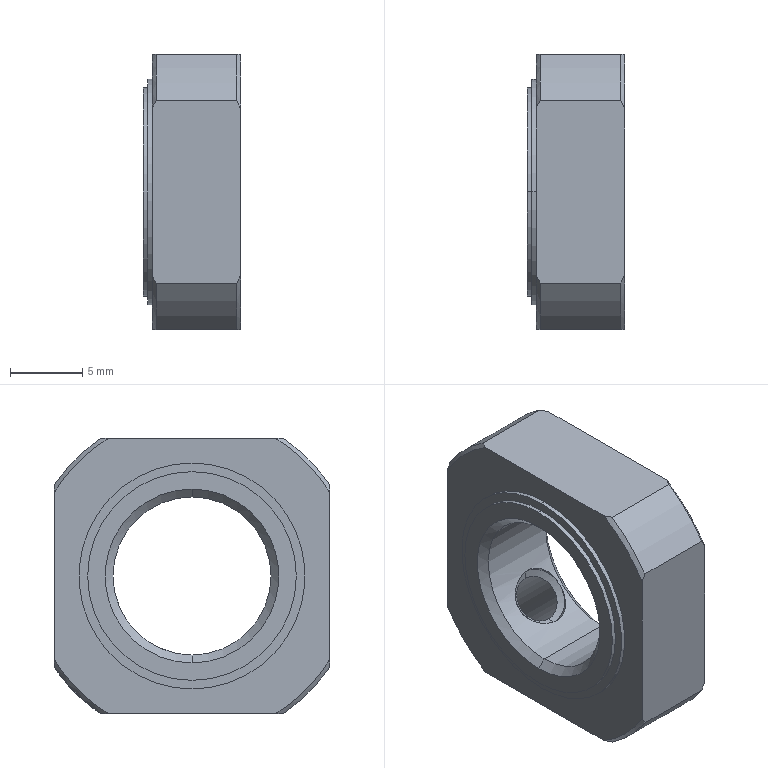Part | STEP file | 12bswnut | 1 solid | 39 faces | box 6.7 x 19 x 19 mm | volume 1510 mm3 | cone 16 | cylinder 15 | plane 8 | commonest cylinder face diameters 22.8 x4 4 x3 3.242 x2 10.917 x2 14.4 x2 15.6 x2
STEP:
#1=CARTESIAN_POINT('',(6.159,0.,-5.458));
#2=VERTEX_POINT('',#1);
#3=CARTESIAN_POINT('',(6.159,0.,5.458));
#4=VERTEX_POINT('',#3);
#5=CARTESIAN_POINT('',(6.159,0.,0.));
#6=DIRECTION('',(-1.,0.,0.));
#7=DIRECTION('',(0.,0.,1.));
#8=AXIS2_PLACEMENT_3D('',#5,#6,#7);
#9=CIRCLE('',#8,5.458);
#10=EDGE_CURVE('',#2,#4,#9,.T.);
#11=ORIENTED_EDGE('',*,*,#10,.T.);
#12=CARTESIAN_POINT('',(6.7,0.,6.));
#13=VERTEX_POINT('',#12);
#14=CARTESIAN_POINT('',(6.7,0.,6.));
#15=DIRECTION('',(0.7071,0.,0.7071));
#16=VECTOR('',#15,1000.);
#17=LINE('',#14,#16);
#18=EDGE_CURVE('',#4,#13,#17,.T.);
#19=ORIENTED_EDGE('',*,*,#18,.T.);
#20=CARTESIAN_POINT('',(6.7,0.,-6.));
#21=VERTEX_POINT('',#20);
#22=CARTESIAN_POINT('',(6.7,0.,0.));
#23=DIRECTION('',(-1.,0.,0.));
#24=DIRECTION('',(0.,0.,1.));
#25=AXIS2_PLACEMENT_3D('',#22,#23,#24);
#26=CIRCLE('',#25,6.);
#27=EDGE_CURVE('',#21,#13,#26,.T.);
#28=ORIENTED_EDGE('',*,*,#27,.F.);
#29=CARTESIAN_POINT('',(6.7,0.,-6.));
#30=DIRECTION('',(0.7071,0.,-0.7071));
#31=VECTOR('',#30,1000.);
#32=LINE('',#29,#31);
#33=EDGE_CURVE('',#2,#21,#32,.T.);
#34=ORIENTED_EDGE('',*,*,#33,.F.);
#35=EDGE_LOOP('',(#11,#19,#28,#34));
#36=FACE_OUTER_BOUND('',#35,.T.);
#37=CARTESIAN_POINT('',(6.7,0.,0.));
#38=DIRECTION('',(1.,0.,0.));
#39=DIRECTION('',(0.,0.,-1.));
#40=AXIS2_PLACEMENT_3D('',#37,#38,#39);
#41=CONICAL_SURFACE('',#40,6.,0.7854);
#42=ADVANCED_FACE('',(#36),#41,.F.);
#43=ORIENTED_EDGE('',*,*,#10,.F.);
#44=CARTESIAN_POINT('',(0.5415,0.,-5.458));
#45=VERTEX_POINT('',#44);
#46=CARTESIAN_POINT('',(6.7,0.,-5.458));
#47=DIRECTION('',(-1.,0.,0.));
#48=VECTOR('',#47,1000.);
#49=LINE('',#46,#48);
#50=EDGE_CURVE('',#2,#45,#49,.T.);
#51=ORIENTED_EDGE('',*,*,#50,.T.);
#52=CARTESIAN_POINT('',(0.5415,0.,5.458));
#53=VERTEX_POINT('',#52);
#54=CARTESIAN_POINT('',(0.5415,0.,0.));
#55=DIRECTION('',(-1.,0.,0.));
#56=DIRECTION('',(0.,0.,1.));
#57=AXIS2_PLACEMENT_3D('',#54,#55,#56);
#58=CIRCLE('',#57,5.458);
#59=EDGE_CURVE('',#45,#53,#58,.T.);
#60=ORIENTED_EDGE('',*,*,#59,.T.);
#61=CARTESIAN_POINT('',(6.7,0.,5.458));
#62=DIRECTION('',(-1.,0.,0.));
#63=VECTOR('',#62,1000.);
#64=LINE('',#61,#63);
#65=EDGE_CURVE('',#4,#53,#64,.T.);
#66=ORIENTED_EDGE('',*,*,#65,.F.);
#67=EDGE_LOOP('',(#43,#51,#60,#66));
#68=FACE_OUTER_BOUND('',#67,.T.);
#69=CARTESIAN_POINT('',(6.7,0.,0.));
#70=DIRECTION('',(-1.,0.,0.));
#71=DIRECTION('',(0.,0.,1.));
#72=AXIS2_PLACEMENT_3D('',#69,#70,#71);
#73=CYLINDRICAL_SURFACE('',#72,5.458);
#74=ADVANCED_FACE('',(#68),#73,.F.);
#75=ORIENTED_EDGE('',*,*,#59,.F.);
#76=CARTESIAN_POINT('',(0.,0.,-6.));
#77=VERTEX_POINT('',#76);
#78=CARTESIAN_POINT('',(0.5415,0.,-5.458));
#79=DIRECTION('',(-0.7071,0.,-0.7071));
#80=VECTOR('',#79,1000.);
#81=LINE('',#78,#80);
#82=EDGE_CURVE('',#45,#77,#81,.T.);
#83=ORIENTED_EDGE('',*,*,#82,.T.);
#84=CARTESIAN_POINT('',(0.,0.,6.));
#85=VERTEX_POINT('',#84);
#86=CARTESIAN_POINT('',(0.,0.,0.));
#87=DIRECTION('',(-1.,0.,0.));
#88=DIRECTION('',(0.,0.,1.));
#89=AXIS2_PLACEMENT_3D('',#86,#87,#88);
#90=CIRCLE('',#89,6.);
#91=EDGE_CURVE('',#77,#85,#90,.T.);
#92=ORIENTED_EDGE('',*,*,#91,.T.);
#93=CARTESIAN_POINT('',(0.5415,0.,5.458));
#94=DIRECTION('',(-0.7071,0.,0.7071));
#95=VECTOR('',#94,1000.);
#96=LINE('',#93,#95);
#97=EDGE_CURVE('',#53,#85,#96,.T.);
#98=ORIENTED_EDGE('',*,*,#97,.F.);
#99=EDGE_LOOP('',(#75,#83,#92,#98));
#100=FACE_OUTER_BOUND('',#99,.T.);
#101=CARTESIAN_POINT('',(0.5415,0.,0.));
#102=DIRECTION('',(-1.,0.,0.));
#103=DIRECTION('',(0.,0.,1.));
#104=AXIS2_PLACEMENT_3D('',#101,#102,#103);
#105=CONICAL_SURFACE('',#104,5.458,0.7854);
#106=ADVANCED_FACE('',(#100),#105,.F.);
#107=CARTESIAN_POINT('',(3.95,2.982,-5.274));
#108=VERTEX_POINT('',#107);
#109=CARTESIAN_POINT('',(3.95,5.274,-2.982));
#110=VERTEX_POINT('',#109);
#111=CARTESIAN_POINT('',(3.95,4.128,-4.128));
#112=DIRECTION('',(0.,0.7071,-0.7071));
#113=DIRECTION('',(0.,0.7071,0.7071));
#114=AXIS2_PLACEMENT_3D('',#111,#112,#113);
#115=CIRCLE('',#114,1.621);
#116=EDGE_CURVE('',#108,#110,#115,.T.);
#117=ORIENTED_EDGE('',*,*,#116,.T.);
#118=CARTESIAN_POINT('',(3.95,5.274,-2.446));
#119=VERTEX_POINT('',#118);
#120=CARTESIAN_POINT('',(3.95,5.274,-2.446));
#121=DIRECTION('',(0.,0.,1.));
#122=VECTOR('',#121,1000.);
#123=LINE('',#120,#122);
#124=EDGE_CURVE('',#110,#119,#123,.T.);
#125=ORIENTED_EDGE('',*,*,#124,.T.);
#126=CARTESIAN_POINT('',(1.95,3.86,-3.86));
#127=VERTEX_POINT('',#126);
#128=CARTESIAN_POINT('',(3.95,3.86,-3.86));
#129=DIRECTION('',(0.,0.7071,-0.7071));
#130=DIRECTION('',(0.,0.7071,0.7071));
#131=AXIS2_PLACEMENT_3D('',#128,#129,#130);
#132=CIRCLE('',#131,2.);
#133=EDGE_CURVE('',#127,#119,#132,.T.);
#134=ORIENTED_EDGE('',*,*,#133,.F.);
#135=CARTESIAN_POINT('',(3.95,2.446,-5.274));
#136=VERTEX_POINT('',#135);
#137=CARTESIAN_POINT('',(3.95,3.86,-3.86));
#138=DIRECTION('',(0.,0.7071,-0.7071));
#139=DIRECTION('',(0.,0.7071,0.7071));
#140=AXIS2_PLACEMENT_3D('',#137,#138,#139);
#141=CIRCLE('',#140,2.);
#142=EDGE_CURVE('',#136,#127,#141,.T.);
#143=ORIENTED_EDGE('',*,*,#142,.F.);
#144=CARTESIAN_POINT('',(3.95,2.446,-5.274));
#145=DIRECTION('',(0.,-1.,0.));
#146=VECTOR('',#145,1000.);
#147=LINE('',#144,#146);
#148=EDGE_CURVE('',#108,#136,#147,.T.);
#149=ORIENTED_EDGE('',*,*,#148,.F.);
#150=EDGE_LOOP('',(#117,#125,#134,#143,#149));
#151=FACE_OUTER_BOUND('',#150,.T.);
#152=CARTESIAN_POINT('',(3.95,3.86,-3.86));
#153=DIRECTION('',(0.,-0.7071,0.7071));
#154=DIRECTION('',(0.,-0.7071,-0.7071));
#155=AXIS2_PLACEMENT_3D('',#152,#153,#154);
#156=CONICAL_SURFACE('',#155,2.,0.7854);
#157=ADVANCED_FACE('',(#151),#156,.F.);
#158=ORIENTED_EDGE('',*,*,#116,.F.);
#159=CARTESIAN_POINT('',(3.95,6.647,-8.939));
#160=VERTEX_POINT('',#159);
#161=CARTESIAN_POINT('',(3.95,-1.146,-1.146));
#162=DIRECTION('',(0.,0.7071,-0.7071));
#163=VECTOR('',#162,1000.);
#164=LINE('',#161,#163);
#165=EDGE_CURVE('',#108,#160,#164,.T.);
#166=ORIENTED_EDGE('',*,*,#165,.T.);
#167=CARTESIAN_POINT('',(3.95,8.939,-6.647));
#168=VERTEX_POINT('',#167);
#169=CARTESIAN_POINT('',(3.95,7.793,-7.793));
#170=DIRECTION('',(0.,0.7071,-0.7071));
#171=DIRECTION('',(0.,0.7071,0.7071));
#172=AXIS2_PLACEMENT_3D('',#169,#170,#171);
#173=CIRCLE('',#172,1.621);
#174=EDGE_CURVE('',#160,#168,#173,.T.);
#175=ORIENTED_EDGE('',*,*,#174,.T.);
#176=CARTESIAN_POINT('',(3.95,1.146,1.146));
#177=DIRECTION('',(0.,0.7071,-0.7071));
#178=VECTOR('',#177,1000.);
#179=LINE('',#176,#178);
#180=EDGE_CURVE('',#110,#168,#179,.T.);
#181=ORIENTED_EDGE('',*,*,#180,.F.);
#182=EDGE_LOOP('',(#158,#166,#175,#181));
#183=FACE_OUTER_BOUND('',#182,.T.);
#184=CARTESIAN_POINT('',(3.95,0.,0.));
#185=DIRECTION('',(0.,0.7071,-0.7071));
#186=DIRECTION('',(0.,0.7071,0.7071));
#187=AXIS2_PLACEMENT_3D('',#184,#185,#186);
#188=CYLINDRICAL_SURFACE('',#187,1.621);
#189=ADVANCED_FACE('',(#183),#188,.F.);
#190=ORIENTED_EDGE('',*,*,#174,.F.);
#191=CARTESIAN_POINT('',(3.95,6.647,-9.262));
#192=VERTEX_POINT('',#191);
#193=CARTESIAN_POINT('',(3.95,6.647,-8.939));
#194=DIRECTION('',(0.,0.,-1.));
#195=VECTOR('',#194,1000.);
#196=LINE('',#193,#195);
#197=EDGE_CURVE('',#160,#192,#196,.T.);
#198=ORIENTED_EDGE('',*,*,#197,.T.);
#199=CARTESIAN_POINT('',(3.95,9.262,-6.647));
#200=VERTEX_POINT('',#199);
#201=CARTESIAN_POINT('',(3.95,6.647,-9.262));
#202=CARTESIAN_POINT('',(3.699,6.647,-9.262));
#203=CARTESIAN_POINT('',(3.445,6.684,-9.235));
#204=CARTESIAN_POINT('',(2.975,6.826,-9.131));
#205=CARTESIAN_POINT('',(2.753,6.932,-9.052));
#206=CARTESIAN_POINT('',(2.471,7.129,-8.896));
#207=CARTESIAN_POINT('',(2.384,7.203,-8.837));
#208=CARTESIAN_POINT('',(2.233,7.358,-8.708));
#209=CARTESIAN_POINT('',(2.168,7.44,-8.638));
#210=CARTESIAN_POINT('',(2.06,7.613,-8.486));
#211=CARTESIAN_POINT('',(2.02,7.702,-8.406));
#212=CARTESIAN_POINT('',(1.964,7.88,-8.239));
#213=CARTESIAN_POINT('',(1.95,7.972,-8.15));
#214=CARTESIAN_POINT('',(1.95,8.15,-7.972));
#215=CARTESIAN_POINT('',(1.964,8.237,-7.882));
#216=CARTESIAN_POINT('',(2.019,8.406,-7.702));
#217=CARTESIAN_POINT('',(2.061,8.487,-7.612));
#218=CARTESIAN_POINT('',(2.167,8.637,-7.441));
#219=CARTESIAN_POINT('',(2.233,8.708,-7.358));
#220=CARTESIAN_POINT('',(2.385,8.837,-7.202));
#221=CARTESIAN_POINT('',(2.47,8.895,-7.13));
#222=CARTESIAN_POINT('',(2.658,9.,-6.998));
#223=CARTESIAN_POINT('',(2.761,9.046,-6.938));
#224=CARTESIAN_POINT('',(2.977,9.124,-6.835));
#225=CARTESIAN_POINT('',(3.09,9.157,-6.791));
#226=CARTESIAN_POINT('',(3.447,9.236,-6.683));
#227=CARTESIAN_POINT('',(3.697,9.262,-6.647));
#228=CARTESIAN_POINT('',(3.95,9.262,-6.647));
#229=B_SPLINE_CURVE_WITH_KNOTS('',3,(#201,#202,#203,#204,#205,#206,#207,#208,#209,#210,#211,#212,#213,#214,#215,#216,#217,#218,#219,#220,#221,#222,#223,#224,#225,#226,#227,#228),.UNSPECIFIED.,.F.,.F.,(4,2,2,2,2,2,2,2,2,2,2,2,2,4),(0.01036,0.01111,0.01187,0.01224,0.01262,0.013,0.01338,0.01375,0.01413,0.01451,0.01489,0.01526,0.01564,0.01639),.UNSPECIFIED.);
#230=EDGE_CURVE('',#192,#200,#229,.T.);
#231=ORIENTED_EDGE('',*,*,#230,.T.);
#232=CARTESIAN_POINT('',(3.95,8.939,-6.647));
#233=DIRECTION('',(0.,1.,0.));
#234=VECTOR('',#233,1000.);
#235=LINE('',#232,#234);
#236=EDGE_CURVE('',#168,#200,#235,.T.);
#237=ORIENTED_EDGE('',*,*,#236,.F.);
#238=EDGE_LOOP('',(#190,#198,#231,#237));
#239=FACE_OUTER_BOUND('',#238,.T.);
#240=CARTESIAN_POINT('',(3.95,7.793,-7.793));
#241=DIRECTION('',(0.,0.7071,-0.7071));
#242=DIRECTION('',(0.,0.7071,0.7071));
#243=AXIS2_PLACEMENT_3D('',#240,#241,#242);
#244=CONICAL_SURFACE('',#243,1.621,0.7854);
#245=ADVANCED_FACE('',(#239),#244,.F.);
#246=CARTESIAN_POINT('',(0.6,0.,7.8));
#247=VERTEX_POINT('',#246);
#248=CARTESIAN_POINT('',(0.6,0.,-7.8));
#249=VERTEX_POINT('',#248);
#250=CARTESIAN_POINT('',(0.6,0.,0.));
#251=DIRECTION('',(-1.,0.,0.));
#252=DIRECTION('',(0.,0.,1.));
#253=AXIS2_PLACEMENT_3D('',#250,#251,#252);
#254=CIRCLE('',#253,7.8);
#255=EDGE_CURVE('',#247,#249,#254,.T.);
#256=ORIENTED_EDGE('',*,*,#255,.T.);
#257=CARTESIAN_POINT('',(0.3,0.,-7.8));
#258=VERTEX_POINT('',#257);
#259=CARTESIAN_POINT('',(6.7,0.,-7.8));
#260=DIRECTION('',(-1.,0.,0.));
#261=VECTOR('',#260,1000.);
#262=LINE('',#259,#261);
#263=EDGE_CURVE('',#249,#258,#262,.T.);
#264=ORIENTED_EDGE('',*,*,#263,.T.);
#265=CARTESIAN_POINT('',(0.3,0.,7.8));
#266=VERTEX_POINT('',#265);
#267=CARTESIAN_POINT('',(0.3,0.,0.));
#268=DIRECTION('',(-1.,0.,0.));
#269=DIRECTION('',(0.,0.,1.));
#270=AXIS2_PLACEMENT_3D('',#267,#268,#269);
#271=CIRCLE('',#270,7.8);
#272=EDGE_CURVE('',#266,#258,#271,.T.);
#273=ORIENTED_EDGE('',*,*,#272,.F.);
#274=CARTESIAN_POINT('',(6.7,0.,7.8));
#275=DIRECTION('',(-1.,0.,0.));
#276=VECTOR('',#275,1000.);
#277=LINE('',#274,#276);
#278=EDGE_CURVE('',#247,#266,#277,.T.);
#279=ORIENTED_EDGE('',*,*,#278,.F.);
#280=EDGE_LOOP('',(#256,#264,#273,#279));
#281=FACE_OUTER_BOUND('',#280,.T.);
#282=CARTESIAN_POINT('',(6.7,0.,0.));
#283=DIRECTION('',(-1.,0.,0.));
#284=DIRECTION('',(0.,0.,1.));
#285=AXIS2_PLACEMENT_3D('',#282,#283,#284);
#286=CYLINDRICAL_SURFACE('',#285,7.8);
#287=ADVANCED_FACE('',(#281),#286,.T.);
#288=CARTESIAN_POINT('',(0.3,0.,7.2));
#289=VERTEX_POINT('',#288);
#290=CARTESIAN_POINT('',(0.3,0.,-7.2));
#291=VERTEX_POINT('',#290);
#292=CARTESIAN_POINT('',(0.3,0.,0.));
#293=DIRECTION('',(-1.,0.,0.));
#294=DIRECTION('',(0.,0.,1.));
#295=AXIS2_PLACEMENT_3D('',#292,#293,#294);
#296=CIRCLE('',#295,7.2);
#297=EDGE_CURVE('',#289,#291,#296,.T.);
#298=ORIENTED_EDGE('',*,*,#297,.T.);
#299=CARTESIAN_POINT('',(0.,0.,-7.2));
#300=VERTEX_POINT('',#299);
#301=CARTESIAN_POINT('',(6.7,0.,-7.2));
#302=DIRECTION('',(-1.,0.,0.));
#303=VECTOR('',#302,1000.);
#304=LINE('',#301,#303);
#305=EDGE_CURVE('',#291,#300,#304,.T.);
#306=ORIENTED_EDGE('',*,*,#305,.T.);
#307=CARTESIAN_POINT('',(0.,0.,7.2));
#308=VERTEX_POINT('',#307);
#309=CARTESIAN_POINT('',(0.,0.,0.));
#310=DIRECTION('',(-1.,0.,0.));
#311=DIRECTION('',(0.,0.,1.));
#312=AXIS2_PLACEMENT_3D('',#309,#310,#311);
#313=CIRCLE('',#312,7.2);
#314=EDGE_CURVE('',#308,#300,#313,.T.);
#315=ORIENTED_EDGE('',*,*,#314,.F.);
#316=CARTESIAN_POINT('',(6.7,0.,7.2));
#317=DIRECTION('',(-1.,0.,0.));
#318=VECTOR('',#317,1000.);
#319=LINE('',#316,#318);
#320=EDGE_CURVE('',#289,#308,#319,.T.);
#321=ORIENTED_EDGE('',*,*,#320,.F.);
#322=EDGE_LOOP('',(#298,#306,#315,#321));
#323=FACE_OUTER_BOUND('',#322,.T.);
#324=CARTESIAN_POINT('',(6.7,0.,0.));
#325=DIRECTION('',(-1.,0.,0.));
#326=DIRECTION('',(0.,0.,1.));
#327=AXIS2_PLACEMENT_3D('',#324,#325,#326);
#328=CYLINDRICAL_SURFACE('',#327,7.2);
#329=ADVANCED_FACE('',(#323),#328,.T.);
#330=CARTESIAN_POINT('',(5.95,3.86,-3.86));
#331=VERTEX_POINT('',#330);
#332=CARTESIAN_POINT('',(3.95,5.006,-2.177));
#333=VERTEX_POINT('',#332);
#334=CARTESIAN_POINT('',(5.95,3.86,-3.86));
#335=CARTESIAN_POINT('',(5.95,3.953,-3.767));
#336=CARTESIAN_POINT('',(5.937,4.042,-3.671));
#337=CARTESIAN_POINT('',(5.885,4.212,-3.474));
#338=CARTESIAN_POINT('',(5.846,4.292,-3.374));
#339=CARTESIAN_POINT('',(5.746,4.438,-3.18));
#340=CARTESIAN_POINT('',(5.683,4.506,-3.083));
#341=CARTESIAN_POINT('',(5.538,4.627,-2.897));
#342=CARTESIAN_POINT('',(5.455,4.681,-2.81));
#343=CARTESIAN_POINT('',(5.272,4.776,-2.645));
#344=CARTESIAN_POINT('',(5.17,4.817,-2.568));
#345=CARTESIAN_POINT('',(4.954,4.886,-2.434));
#346=CARTESIAN_POINT('',(4.84,4.915,-2.375));
#347=CARTESIAN_POINT('',(4.598,4.961,-2.278));
#348=CARTESIAN_POINT('',(4.471,4.978,-2.24));
#349=CARTESIAN_POINT('',(4.214,5.,-2.19));
#350=CARTESIAN_POINT('',(4.083,5.006,-2.177));
#351=CARTESIAN_POINT('',(3.95,5.006,-2.177));
#352=B_SPLINE_CURVE_WITH_KNOTS('',3,(#334,#335,#336,#337,#338,#339,#340,#341,#342,#343,#344,#345,#346,#347,#348,#349,#350,#351),.UNSPECIFIED.,.F.,.F.,(4,2,2,2,2,2,2,2,4),(0.009461,0.009855,0.01025,0.01064,0.01104,0.01143,0.01183,0.01222,0.01261),.UNSPECIFIED.);
#353=EDGE_CURVE('',#331,#333,#352,.T.);
#354=ORIENTED_EDGE('',*,*,#353,.T.);
#355=CARTESIAN_POINT('',(3.95,1.414,1.414));
#356=DIRECTION('',(0.,0.7071,-0.7071));
#357=VECTOR('',#356,1000.);
#358=LINE('',#355,#357);
#359=EDGE_CURVE('',#333,#119,#358,.T.);
#360=ORIENTED_EDGE('',*,*,#359,.T.);
#361=CARTESIAN_POINT('',(3.95,3.86,-3.86));
#362=DIRECTION('',(0.,0.7071,-0.7071));
#363=DIRECTION('',(0.,0.7071,0.7071));
#364=AXIS2_PLACEMENT_3D('',#361,#362,#363);
#365=CIRCLE('',#364,2.);
#366=EDGE_CURVE('',#119,#331,#365,.T.);
#367=ORIENTED_EDGE('',*,*,#366,.T.);
#368=EDGE_LOOP('',(#354,#360,#367));
#369=FACE_OUTER_BOUND('',#368,.T.);
#370=CARTESIAN_POINT('',(3.95,0.,0.));
#371=DIRECTION('',(0.,0.7071,-0.7071));
#372=DIRECTION('',(0.,0.7071,0.7071));
#373=AXIS2_PLACEMENT_3D('',#370,#371,#372);
#374=CYLINDRICAL_SURFACE('',#373,2.);
#375=ADVANCED_FACE('',(#369),#374,.F.);
#376=ORIENTED_EDGE('',*,*,#314,.T.);
#377=CARTESIAN_POINT('',(0.,0.,0.));
#378=DIRECTION('',(-1.,0.,0.));
#379=DIRECTION('',(0.,0.,1.));
#380=AXIS2_PLACEMENT_3D('',#377,#378,#379);
#381=CIRCLE('',#380,7.2);
#382=EDGE_CURVE('',#300,#308,#381,.T.);
#383=ORIENTED_EDGE('',*,*,#382,.T.);
#384=EDGE_LOOP('',(#376,#383));
#385=FACE_OUTER_BOUND('',#384,.T.);
#386=CARTESIAN_POINT('',(0.,0.,0.));
#387=DIRECTION('',(-1.,0.,0.));
#388=DIRECTION('',(0.,0.,1.));
#389=AXIS2_PLACEMENT_3D('',#386,#387,#388);
#390=CIRCLE('',#389,6.);
#391=EDGE_CURVE('',#85,#77,#390,.T.);
#392=ORIENTED_EDGE('',*,*,#391,.F.);
#393=ORIENTED_EDGE('',*,*,#91,.F.);
#394=EDGE_LOOP('',(#392,#393));
#395=FACE_BOUND('',#394,.T.);
#396=CARTESIAN_POINT('',(0.,0.,0.));
#397=DIRECTION('',(1.,0.,0.));
#398=DIRECTION('',(0.,0.,-1.));
#399=AXIS2_PLACEMENT_3D('',#396,#397,#398);
#400=PLANE('',#399);
#401=ADVANCED_FACE('',(#385,#395),#400,.F.);
#402=CARTESIAN_POINT('',(6.7,5.789,9.5));
#403=VERTEX_POINT('',#402);
#404=CARTESIAN_POINT('',(6.7,9.5,5.789));
#405=VERTEX_POINT('',#404);
#406=CARTESIAN_POINT('',(6.7,0.,0.));
#407=DIRECTION('',(-1.,0.,0.));
#408=DIRECTION('',(0.,0.,1.));
#409=AXIS2_PLACEMENT_3D('',#406,#407,#408);
#410=CIRCLE('',#409,11.125);
#411=EDGE_CURVE('',#403,#405,#410,.T.);
#412=ORIENTED_EDGE('',*,*,#411,.F.);
#413=CARTESIAN_POINT('',(6.7,-5.789,9.5));
#414=VERTEX_POINT('',#413);
#415=CARTESIAN_POINT('',(6.7,11.125,9.5));
#416=DIRECTION('',(0.,-1.,0.));
#417=VECTOR('',#416,1000.);
#418=LINE('',#415,#417);
#419=EDGE_CURVE('',#403,#414,#418,.T.);
#420=ORIENTED_EDGE('',*,*,#419,.T.);
#421=CARTESIAN_POINT('',(6.7,-9.5,5.789));
#422=VERTEX_POINT('',#421);
#423=CARTESIAN_POINT('',(6.7,0.,0.));
#424=DIRECTION('',(-1.,0.,0.));
#425=DIRECTION('',(0.,0.,1.));
#426=AXIS2_PLACEMENT_3D('',#423,#424,#425);
#427=CIRCLE('',#426,11.125);
#428=EDGE_CURVE('',#422,#414,#427,.T.);
#429=ORIENTED_EDGE('',*,*,#428,.F.);
#430=CARTESIAN_POINT('',(6.7,-9.5,-5.789));
#431=VERTEX_POINT('',#430);
#432=CARTESIAN_POINT('',(6.7,-9.5,0.));
#433=DIRECTION('',(0.,0.,-1.));
#434=VECTOR('',#433,1000.);
#435=LINE('',#432,#434);
#436=EDGE_CURVE('',#422,#431,#435,.T.);
#437=ORIENTED_EDGE('',*,*,#436,.T.);
#438=CARTESIAN_POINT('',(6.7,-5.789,-9.5));
#439=VERTEX_POINT('',#438);
#440=CARTESIAN_POINT('',(6.7,0.,0.));
#441=DIRECTION('',(-1.,0.,0.));
#442=DIRECTION('',(0.,0.,1.));
#443=AXIS2_PLACEMENT_3D('',#440,#441,#442);
#444=CIRCLE('',#443,11.125);
#445=EDGE_CURVE('',#439,#431,#444,.T.);
#446=ORIENTED_EDGE('',*,*,#445,.F.);
#447=CARTESIAN_POINT('',(6.7,5.789,-9.5));
#448=VERTEX_POINT('',#447);
#449=CARTESIAN_POINT('',(6.7,11.125,-9.5));
#450=DIRECTION('',(0.,1.,0.));
#451=VECTOR('',#450,1000.);
#452=LINE('',#449,#451);
#453=EDGE_CURVE('',#439,#448,#452,.T.);
#454=ORIENTED_EDGE('',*,*,#453,.T.);
#455=CARTESIAN_POINT('',(6.7,9.5,-5.789));
#456=VERTEX_POINT('',#455);
#457=CARTESIAN_POINT('',(6.7,0.,0.));
#458=DIRECTION('',(-1.,0.,0.));
#459=DIRECTION('',(0.,0.,1.));
#460=AXIS2_PLACEMENT_3D('',#457,#458,#459);
#461=CIRCLE('',#460,11.125);
#462=EDGE_CURVE('',#456,#448,#461,.T.);
#463=ORIENTED_EDGE('',*,*,#462,.F.);
#464=CARTESIAN_POINT('',(6.7,9.5,0.));
#465=DIRECTION('',(0.,0.,1.));
#466=VECTOR('',#465,1000.);
#467=LINE('',#464,#466);
#468=EDGE_CURVE('',#456,#405,#467,.T.);
#469=ORIENTED_EDGE('',*,*,#468,.T.);
#470=EDGE_LOOP('',(#412,#420,#429,#437,#446,#454,#463,#469));
#471=FACE_OUTER_BOUND('',#470,.T.);
#472=ORIENTED_EDGE('',*,*,#27,.T.);
#473=CARTESIAN_POINT('',(6.7,0.,0.));
#474=DIRECTION('',(-1.,0.,0.));
#475=DIRECTION('',(0.,0.,1.));
#476=AXIS2_PLACEMENT_3D('',#473,#474,#475);
#477=CIRCLE('',#476,6.);
#478=EDGE_CURVE('',#13,#21,#477,.T.);
#479=ORIENTED_EDGE('',*,*,#478,.T.);
#480=EDGE_LOOP('',(#472,#479));
#481=FACE_BOUND('',#480,.T.);
#482=CARTESIAN_POINT('',(6.7,11.125,0.));
#483=DIRECTION('',(-1.,0.,0.));
#484=DIRECTION('',(0.,0.,1.));
#485=AXIS2_PLACEMENT_3D('',#482,#483,#484);
#486=PLANE('',#485);
#487=ADVANCED_FACE('',(#471,#481),#486,.F.);
#488=CARTESIAN_POINT('',(3.95,3.86,-3.86));
#489=DIRECTION('',(0.,0.7071,-0.7071));
#490=DIRECTION('',(0.,0.7071,0.7071));
#491=AXIS2_PLACEMENT_3D('',#488,#489,#490);
#492=CIRCLE('',#491,2.);
#493=EDGE_CURVE('',#331,#136,#492,.T.);
#494=ORIENTED_EDGE('',*,*,#493,.T.);
#495=ORIENTED_EDGE('',*,*,#142,.T.);
#496=CARTESIAN_POINT('',(1.95,3.86,-3.86));
#497=CARTESIAN_POINT('',(1.95,3.767,-3.953));
#498=CARTESIAN_POINT('',(1.963,3.669,-4.044));
#499=CARTESIAN_POINT('',(2.015,3.473,-4.213));
#500=CARTESIAN_POINT('',(2.053,3.375,-4.292));
#501=CARTESIAN_POINT('',(2.155,3.178,-4.44));
#502=CARTESIAN_POINT('',(2.217,3.082,-4.506));
#503=CARTESIAN_POINT('',(2.362,2.898,-4.627));
#504=CARTESIAN_POINT('',(2.445,2.809,-4.681));
#505=CARTESIAN_POINT('',(2.629,2.644,-4.776));
#506=CARTESIAN_POINT('',(2.729,2.569,-4.817));
#507=CARTESIAN_POINT('',(2.945,2.434,-4.886));
#508=CARTESIAN_POINT('',(3.061,2.375,-4.915));
#509=CARTESIAN_POINT('',(3.302,2.278,-4.961));
#510=CARTESIAN_POINT('',(3.427,2.241,-4.977));
#511=CARTESIAN_POINT('',(3.686,2.19,-5.));
#512=CARTESIAN_POINT('',(3.818,2.177,-5.006));
#513=CARTESIAN_POINT('',(4.081,2.177,-5.006));
#514=CARTESIAN_POINT('',(4.214,2.19,-5.));
#515=CARTESIAN_POINT('',(4.473,2.241,-4.977));
#516=CARTESIAN_POINT('',(4.598,2.278,-4.961));
#517=CARTESIAN_POINT('',(4.84,2.375,-4.915));
#518=CARTESIAN_POINT('',(4.956,2.435,-4.886));
#519=CARTESIAN_POINT('',(5.172,2.569,-4.817));
#520=CARTESIAN_POINT('',(5.272,2.645,-4.776));
#521=CARTESIAN_POINT('',(5.457,2.811,-4.68));
#522=CARTESIAN_POINT('',(5.539,2.899,-4.626));
#523=CARTESIAN_POINT('',(5.683,3.083,-4.506));
#524=CARTESIAN_POINT('',(5.746,3.18,-4.439));
#525=CARTESIAN_POINT('',(5.847,3.375,-4.291));
#526=CARTESIAN_POINT('',(5.885,3.473,-4.213));
#527=CARTESIAN_POINT('',(5.937,3.668,-4.044));
#528=CARTESIAN_POINT('',(5.95,3.767,-3.953));
#529=CARTESIAN_POINT('',(5.95,3.86,-3.86));
#530=B_SPLINE_CURVE_WITH_KNOTS('',3,(#496,#497,#498,#499,#500,#501,#502,#503,#504,#505,#506,#507,#508,#509,#510,#511,#512,#513,#514,#515,#516,#517,#518,#519,#520,#521,#522,#523,#524,#525,#526,#527,#528,#529),.UNSPECIFIED.,.F.,.F.,(4,2,2,2,2,2,2,2,2,2,2,2,2,2,2,2,4),(0.003155,0.003549,0.003943,0.004337,0.004731,0.005126,0.00552,0.005914,0.006308,0.006702,0.007096,0.00749,0.007884,0.008278,0.008672,0.009067,0.009461),.UNSPECIFIED.);
#531=EDGE_CURVE('',#127,#331,#530,.T.);
#532=ORIENTED_EDGE('',*,*,#531,.T.);
#533=EDGE_LOOP('',(#494,#495,#532));
#534=FACE_OUTER_BOUND('',#533,.T.);
#535=CARTESIAN_POINT('',(3.95,0.,0.));
#536=DIRECTION('',(0.,0.7071,-0.7071));
#537=DIRECTION('',(0.,0.7071,0.7071));
#538=AXIS2_PLACEMENT_3D('',#535,#536,#537);
#539=CYLINDRICAL_SURFACE('',#538,2.);
#540=ADVANCED_FACE('',(#534),#539,.F.);
#541=ORIENTED_EDGE('',*,*,#359,.F.);
#542=CARTESIAN_POINT('',(3.95,5.006,-2.177));
#543=CARTESIAN_POINT('',(3.817,5.006,-2.177));
#544=CARTESIAN_POINT('',(3.686,5.,-2.19));
#545=CARTESIAN_POINT('',(3.428,4.977,-2.241));
#546=CARTESIAN_POINT('',(3.301,4.96,-2.279));
#547=CARTESIAN_POINT('',(3.059,4.915,-2.376));
#548=CARTESIAN_POINT('',(2.945,4.886,-2.434));
#549=CARTESIAN_POINT('',(2.728,4.816,-2.57));
#550=CARTESIAN_POINT('',(2.627,4.775,-2.646));
#551=CARTESIAN_POINT('',(2.353,4.633,-2.892));
#552=CARTESIAN_POINT('',(2.204,4.511,-3.083));
#553=CARTESIAN_POINT('',(2.054,4.292,-3.375));
#554=CARTESIAN_POINT('',(2.015,4.212,-3.475));
#555=CARTESIAN_POINT('',(1.963,4.042,-3.671));
#556=CARTESIAN_POINT('',(1.95,3.953,-3.767));
#557=CARTESIAN_POINT('',(1.95,3.86,-3.86));
#558=B_SPLINE_CURVE_WITH_KNOTS('',3,(#542,#543,#544,#545,#546,#547,#548,#549,#550,#551,#552,#553,#554,#555,#556,#557),.UNSPECIFIED.,.F.,.F.,(4,2,2,2,2,2,2,4),(0.,0.0003944,0.0007888,0.001183,0.001578,0.002366,0.002761,0.003155),.UNSPECIFIED.);
#559=EDGE_CURVE('',#333,#127,#558,.T.);
#560=ORIENTED_EDGE('',*,*,#559,.T.);
#561=ORIENTED_EDGE('',*,*,#133,.T.);
#562=EDGE_LOOP('',(#541,#560,#561));
#563=FACE_OUTER_BOUND('',#562,.T.);
#564=CARTESIAN_POINT('',(3.95,0.,0.));
#565=DIRECTION('',(0.,0.7071,-0.7071));
#566=DIRECTION('',(0.,0.7071,0.7071));
#567=AXIS2_PLACEMENT_3D('',#564,#565,#566);
#568=CYLINDRICAL_SURFACE('',#567,2.);
#569=ADVANCED_FACE('',(#563),#568,.F.);
#570=CARTESIAN_POINT('',(6.425,9.5,-6.302));
#571=VERTEX_POINT('',#570);
#572=CARTESIAN_POINT('',(6.425,6.302,-9.5));
#573=VERTEX_POINT('',#572);
#574=CARTESIAN_POINT('',(6.425,0.,0.));
#575=DIRECTION('',(-1.,0.,0.));
#576=DIRECTION('',(0.,0.,1.));
#577=AXIS2_PLACEMENT_3D('',#574,#575,#576);
#578=CIRCLE('',#577,11.4);
#579=EDGE_CURVE('',#571,#573,#578,.T.);
#580=ORIENTED_EDGE('',*,*,#579,.T.);
#581=CARTESIAN_POINT('',(0.875,6.302,-9.5));
#582=VERTEX_POINT('',#581);
#583=CARTESIAN_POINT('',(6.7,6.302,-9.5));
#584=DIRECTION('',(-1.,0.,0.));
#585=VECTOR('',#584,1000.);
#586=LINE('',#583,#585);
#587=EDGE_CURVE('',#573,#582,#586,.T.);
#588=ORIENTED_EDGE('',*,*,#587,.T.);
#589=CARTESIAN_POINT('',(0.875,9.5,-6.302));
#590=VERTEX_POINT('',#589);
#591=CARTESIAN_POINT('',(0.875,0.,0.));
#592=DIRECTION('',(-1.,0.,0.));
#593=DIRECTION('',(0.,0.,1.));
#594=AXIS2_PLACEMENT_3D('',#591,#592,#593);
#595=CIRCLE('',#594,11.4);
#596=EDGE_CURVE('',#590,#582,#595,.T.);
#597=ORIENTED_EDGE('',*,*,#596,.F.);
#598=CARTESIAN_POINT('',(6.7,9.5,-6.302));
#599=DIRECTION('',(1.,0.,0.));
#600=VECTOR('',#599,1000.);
#601=LINE('',#598,#600);
#602=EDGE_CURVE('',#590,#571,#601,.T.);
#603=ORIENTED_EDGE('',*,*,#602,.T.);
#604=EDGE_LOOP('',(#580,#588,#597,#603));
#605=FACE_OUTER_BOUND('',#604,.T.);
#606=CARTESIAN_POINT('',(3.95,9.262,-6.647));
#607=CARTESIAN_POINT('',(4.077,9.262,-6.647));
#608=CARTESIAN_POINT('',(4.202,9.255,-6.656));
#609=CARTESIAN_POINT('',(4.449,9.229,-6.692));
#610=CARTESIAN_POINT('',(4.572,9.209,-6.719));
#611=CARTESIAN_POINT('',(4.809,9.157,-6.791));
#612=CARTESIAN_POINT('',(4.922,9.125,-6.834));
#613=CARTESIAN_POINT('',(5.137,9.047,-6.937));
#614=CARTESIAN_POINT('',(5.24,9.,-6.997));
#615=CARTESIAN_POINT('',(5.428,8.896,-7.129));
#616=CARTESIAN_POINT('',(5.513,8.838,-7.201));
#617=CARTESIAN_POINT('',(5.665,8.71,-7.355));
#618=CARTESIAN_POINT('',(5.731,8.639,-7.439));
#619=CARTESIAN_POINT('',(5.838,8.489,-7.61));
#620=CARTESIAN_POINT('',(5.879,8.409,-7.698));
#621=CARTESIAN_POINT('',(5.935,8.24,-7.878));
#622=CARTESIAN_POINT('',(5.95,8.152,-7.97));
#623=CARTESIAN_POINT('',(5.95,7.975,-8.147));
#624=CARTESIAN_POINT('',(5.936,7.883,-8.236));
#625=CARTESIAN_POINT('',(5.881,7.703,-8.405));
#626=CARTESIAN_POINT('',(5.84,7.615,-8.485));
#627=CARTESIAN_POINT('',(5.68,7.356,-8.712));
#628=CARTESIAN_POINT('',(5.525,7.197,-8.843));
#629=CARTESIAN_POINT('',(5.242,6.998,-9.));
#630=CARTESIAN_POINT('',(5.14,6.939,-9.045));
#631=CARTESIAN_POINT('',(4.924,6.835,-9.124));
#632=CARTESIAN_POINT('',(4.809,6.791,-9.157));
#633=CARTESIAN_POINT('',(4.573,6.719,-9.209));
#634=CARTESIAN_POINT('',(4.452,6.692,-9.229));
#635=CARTESIAN_POINT('',(4.203,6.656,-9.255));
#636=CARTESIAN_POINT('',(4.076,6.647,-9.262));
#637=CARTESIAN_POINT('',(3.95,6.647,-9.262));
#638=B_SPLINE_CURVE_WITH_KNOTS('',3,(#606,#607,#608,#609,#610,#611,#612,#613,#614,#615,#616,#617,#618,#619,#620,#621,#622,#623,#624,#625,#626,#627,#628,#629,#630,#631,#632,#633,#634,#635,#636,#637),.UNSPECIFIED.,.F.,.F.,(4,2,2,2,2,2,2,2,2,2,2,2,2,2,2,4),(0.004319,0.004697,0.005074,0.005452,0.005829,0.006207,0.006584,0.006962,0.007339,0.007716,0.008094,0.008849,0.009226,0.009604,0.009981,0.01036),.UNSPECIFIED.);
#639=EDGE_CURVE('',#200,#192,#638,.T.);
#640=ORIENTED_EDGE('',*,*,#639,.F.);
#641=ORIENTED_EDGE('',*,*,#230,.F.);
#642=EDGE_LOOP('',(#640,#641));
#643=FACE_BOUND('',#642,.T.);
#644=CARTESIAN_POINT('',(6.7,0.,0.));
#645=DIRECTION('',(-1.,0.,0.));
#646=DIRECTION('',(0.,0.,1.));
#647=AXIS2_PLACEMENT_3D('',#644,#645,#646);
#648=CYLINDRICAL_SURFACE('',#647,11.4);
#649=ADVANCED_FACE('',(#605,#643),#648,.T.);
#650=CARTESIAN_POINT('',(0.875,-9.5,6.302));
#651=VERTEX_POINT('',#650);
#652=CARTESIAN_POINT('',(0.875,-6.302,9.5));
#653=VERTEX_POINT('',#652);
#654=CARTESIAN_POINT('',(0.875,0.,0.));
#655=DIRECTION('',(-1.,0.,0.));
#656=DIRECTION('',(0.,0.,1.));
#657=AXIS2_PLACEMENT_3D('',#654,#655,#656);
#658=CIRCLE('',#657,11.4);
#659=EDGE_CURVE('',#651,#653,#658,.T.);
#660=ORIENTED_EDGE('',*,*,#659,.T.);
#661=CARTESIAN_POINT('',(0.6,-5.789,9.5));
#662=VERTEX_POINT('',#661);
#663=CARTESIAN_POINT('',(0.875,-6.302,9.5));
#664=CARTESIAN_POINT('',(0.7811,-6.132,9.5));
#665=CARTESIAN_POINT('',(0.6894,-5.961,9.5));
#666=CARTESIAN_POINT('',(0.6,-5.789,9.5));
#667=B_SPLINE_CURVE_WITH_KNOTS('',3,(#663,#664,#665,#666),.UNSPECIFIED.,.F.,.F.,(4,4),(0.01843,0.01901),.UNSPECIFIED.);
#668=EDGE_CURVE('',#653,#662,#667,.T.);
#669=ORIENTED_EDGE('',*,*,#668,.T.);
#670=CARTESIAN_POINT('',(0.6,-9.5,5.789));
#671=VERTEX_POINT('',#670);
#672=CARTESIAN_POINT('',(0.6,0.,0.));
#673=DIRECTION('',(-1.,0.,0.));
#674=DIRECTION('',(0.,0.,1.));
#675=AXIS2_PLACEMENT_3D('',#672,#673,#674);
#676=CIRCLE('',#675,11.125);
#677=EDGE_CURVE('',#671,#662,#676,.T.);
#678=ORIENTED_EDGE('',*,*,#677,.F.);
#679=CARTESIAN_POINT('',(0.6,-9.5,5.789));
#680=CARTESIAN_POINT('',(0.6896,-9.5,5.961));
#681=CARTESIAN_POINT('',(0.7813,-9.5,6.132));
#682=CARTESIAN_POINT('',(0.875,-9.5,6.302));
#683=B_SPLINE_CURVE_WITH_KNOTS('',3,(#679,#680,#681,#682),.UNSPECIFIED.,.F.,.F.,(4,4),(0.03115,0.03173),.UNSPECIFIED.);
#684=EDGE_CURVE('',#671,#651,#683,.T.);
#685=ORIENTED_EDGE('',*,*,#684,.T.);
#686=EDGE_LOOP('',(#660,#669,#678,#685));
#687=FACE_OUTER_BOUND('',#686,.T.);
#688=CARTESIAN_POINT('',(0.875,0.,0.));
#689=DIRECTION('',(1.,0.,0.));
#690=DIRECTION('',(0.,0.,-1.));
#691=AXIS2_PLACEMENT_3D('',#688,#689,#690);
#692=CONICAL_SURFACE('',#691,11.4,0.7854);
#693=ADVANCED_FACE('',(#687),#692,.T.);
#694=CARTESIAN_POINT('',(0.875,-6.302,-9.5));
#695=VERTEX_POINT('',#694);
#696=CARTESIAN_POINT('',(0.875,-9.5,-6.302));
#697=VERTEX_POINT('',#696);
#698=CARTESIAN_POINT('',(0.875,0.,0.));
#699=DIRECTION('',(-1.,0.,0.));
#700=DIRECTION('',(0.,0.,1.));
#701=AXIS2_PLACEMENT_3D('',#698,#699,#700);
#702=CIRCLE('',#701,11.4);
#703=EDGE_CURVE('',#695,#697,#702,.T.);
#704=ORIENTED_EDGE('',*,*,#703,.T.);
#705=CARTESIAN_POINT('',(0.6,-9.5,-5.789));
#706=VERTEX_POINT('',#705);
#707=CARTESIAN_POINT('',(0.875,-9.5,-6.302));
#708=CARTESIAN_POINT('',(0.7811,-9.5,-6.132));
#709=CARTESIAN_POINT('',(0.6894,-9.5,-5.961));
#710=CARTESIAN_POINT('',(0.6,-9.5,-5.789));
#711=B_SPLINE_CURVE_WITH_KNOTS('',3,(#707,#708,#709,#710),.UNSPECIFIED.,.F.,.F.,(4,4),(0.01843,0.01901),.UNSPECIFIED.);
#712=EDGE_CURVE('',#697,#706,#711,.T.);
#713=ORIENTED_EDGE('',*,*,#712,.T.);
#714=CARTESIAN_POINT('',(0.6,-5.789,-9.5));
#715=VERTEX_POINT('',#714);
#716=CARTESIAN_POINT('',(0.6,0.,0.));
#717=DIRECTION('',(-1.,0.,0.));
#718=DIRECTION('',(0.,0.,1.));
#719=AXIS2_PLACEMENT_3D('',#716,#717,#718);
#720=CIRCLE('',#719,11.125);
#721=EDGE_CURVE('',#715,#706,#720,.T.);
#722=ORIENTED_EDGE('',*,*,#721,.F.);
#723=CARTESIAN_POINT('',(0.6,-5.789,-9.5));
#724=CARTESIAN_POINT('',(0.6896,-5.961,-9.5));
#725=CARTESIAN_POINT('',(0.7813,-6.132,-9.5));
#726=CARTESIAN_POINT('',(0.875,-6.302,-9.5));
#727=B_SPLINE_CURVE_WITH_KNOTS('',3,(#723,#724,#725,#726),.UNSPECIFIED.,.F.,.F.,(4,4),(0.03115,0.03173),.UNSPECIFIED.);
#728=EDGE_CURVE('',#715,#695,#727,.T.);
#729=ORIENTED_EDGE('',*,*,#728,.T.);
#730=EDGE_LOOP('',(#704,#713,#722,#729));
#731=FACE_OUTER_BOUND('',#730,.T.);
#732=CARTESIAN_POINT('',(0.875,0.,0.));
#733=DIRECTION('',(1.,0.,0.));
#734=DIRECTION('',(0.,0.,-1.));
#735=AXIS2_PLACEMENT_3D('',#732,#733,#734);
#736=CONICAL_SURFACE('',#735,11.4,0.7854);
#737=ADVANCED_FACE('',(#731),#736,.T.);
#738=ORIENTED_EDGE('',*,*,#596,.T.);
#739=CARTESIAN_POINT('',(0.6,5.789,-9.5));
#740=VERTEX_POINT('',#739);
#741=CARTESIAN_POINT('',(0.875,6.302,-9.5));
#742=CARTESIAN_POINT('',(0.7811,6.132,-9.5));
#743=CARTESIAN_POINT('',(0.6894,5.961,-9.5));
#744=CARTESIAN_POINT('',(0.6,5.789,-9.5));
#745=B_SPLINE_CURVE_WITH_KNOTS('',3,(#741,#742,#743,#744),.UNSPECIFIED.,.F.,.F.,(4,4),(0.01843,0.01901),.UNSPECIFIED.);
#746=EDGE_CURVE('',#582,#740,#745,.T.);
#747=ORIENTED_EDGE('',*,*,#746,.T.);
#748=CARTESIAN_POINT('',(0.6,9.5,-5.789));
#749=VERTEX_POINT('',#748);
#750=CARTESIAN_POINT('',(0.6,0.,0.));
#751=DIRECTION('',(-1.,0.,0.));
#752=DIRECTION('',(0.,0.,1.));
#753=AXIS2_PLACEMENT_3D('',#750,#751,#752);
#754=CIRCLE('',#753,11.125);
#755=EDGE_CURVE('',#749,#740,#754,.T.);
#756=ORIENTED_EDGE('',*,*,#755,.F.);
#757=CARTESIAN_POINT('',(0.6,9.5,-5.789));
#758=CARTESIAN_POINT('',(0.6896,9.5,-5.961));
#759=CARTESIAN_POINT('',(0.7813,9.5,-6.132));
#760=CARTESIAN_POINT('',(0.875,9.5,-6.302));
#761=B_SPLINE_CURVE_WITH_KNOTS('',3,(#757,#758,#759,#760),.UNSPECIFIED.,.F.,.F.,(4,4),(0.03115,0.03173),.UNSPECIFIED.);
#762=EDGE_CURVE('',#749,#590,#761,.T.);
#763=ORIENTED_EDGE('',*,*,#762,.T.);
#764=EDGE_LOOP('',(#738,#747,#756,#763));
#765=FACE_OUTER_BOUND('',#764,.T.);
#766=CARTESIAN_POINT('',(0.875,0.,0.));
#767=DIRECTION('',(1.,0.,0.));
#768=DIRECTION('',(0.,0.,-1.));
#769=AXIS2_PLACEMENT_3D('',#766,#767,#768);
#770=CONICAL_SURFACE('',#769,11.4,0.7854);
#771=ADVANCED_FACE('',(#765),#770,.T.);
#772=CARTESIAN_POINT('',(6.425,-9.5,6.302));
#773=VERTEX_POINT('',#772);
#774=CARTESIAN_POINT('',(6.425,-6.302,9.5));
#775=VERTEX_POINT('',#774);
#776=CARTESIAN_POINT('',(6.425,0.,0.));
#777=DIRECTION('',(-1.,0.,0.));
#778=DIRECTION('',(0.,0.,1.));
#779=AXIS2_PLACEMENT_3D('',#776,#777,#778);
#780=CIRCLE('',#779,11.4);
#781=EDGE_CURVE('',#773,#775,#780,.T.);
#782=ORIENTED_EDGE('',*,*,#781,.T.);
#783=CARTESIAN_POINT('',(6.7,-6.302,9.5));
#784=DIRECTION('',(-1.,0.,0.));
#785=VECTOR('',#784,1000.);
#786=LINE('',#783,#785);
#787=EDGE_CURVE('',#775,#653,#786,.T.);
#788=ORIENTED_EDGE('',*,*,#787,.T.);
#789=ORIENTED_EDGE('',*,*,#659,.F.);
#790=CARTESIAN_POINT('',(6.7,-9.5,6.302));
#791=DIRECTION('',(1.,0.,0.));
#792=VECTOR('',#791,1000.);
#793=LINE('',#790,#792);
#794=EDGE_CURVE('',#651,#773,#793,.T.);
#795=ORIENTED_EDGE('',*,*,#794,.T.);
#796=EDGE_LOOP('',(#782,#788,#789,#795));
#797=FACE_OUTER_BOUND('',#796,.T.);
#798=CARTESIAN_POINT('',(6.7,0.,0.));
#799=DIRECTION('',(-1.,0.,0.));
#800=DIRECTION('',(0.,0.,1.));
#801=AXIS2_PLACEMENT_3D('',#798,#799,#800);
#802=CYLINDRICAL_SURFACE('',#801,11.4);
#803=ADVANCED_FACE('',(#797),#802,.T.);
#804=CARTESIAN_POINT('',(6.425,-6.302,-9.5));
#805=VERTEX_POINT('',#804);
#806=CARTESIAN_POINT('',(6.425,-9.5,-6.302));
#807=VERTEX_POINT('',#806);
#808=CARTESIAN_POINT('',(6.425,0.,0.));
#809=DIRECTION('',(-1.,0.,0.));
#810=DIRECTION('',(0.,0.,1.));
#811=AXIS2_PLACEMENT_3D('',#808,#809,#810);
#812=CIRCLE('',#811,11.4);
#813=EDGE_CURVE('',#805,#807,#812,.T.);
#814=ORIENTED_EDGE('',*,*,#813,.T.);
#815=CARTESIAN_POINT('',(6.7,-9.5,-6.302));
#816=DIRECTION('',(-1.,0.,0.));
#817=VECTOR('',#816,1000.);
#818=LINE('',#815,#817);
#819=EDGE_CURVE('',#807,#697,#818,.T.);
#820=ORIENTED_EDGE('',*,*,#819,.T.);
#821=ORIENTED_EDGE('',*,*,#703,.F.);
#822=CARTESIAN_POINT('',(6.7,-6.302,-9.5));
#823=DIRECTION('',(1.,0.,0.));
#824=VECTOR('',#823,1000.);
#825=LINE('',#822,#824);
#826=EDGE_CURVE('',#695,#805,#825,.T.);
#827=ORIENTED_EDGE('',*,*,#826,.T.);
#828=EDGE_LOOP('',(#814,#820,#821,#827));
#829=FACE_OUTER_BOUND('',#828,.T.);
#830=CARTESIAN_POINT('',(6.7,0.,0.));
#831=DIRECTION('',(-1.,0.,0.));
#832=DIRECTION('',(0.,0.,1.));
#833=AXIS2_PLACEMENT_3D('',#830,#831,#832);
#834=CYLINDRICAL_SURFACE('',#833,11.4);
#835=ADVANCED_FACE('',(#829),#834,.T.);
#836=CARTESIAN_POINT('',(6.425,6.302,9.5));
#837=VERTEX_POINT('',#836);
#838=CARTESIAN_POINT('',(6.425,9.5,6.302));
#839=VERTEX_POINT('',#838);
#840=CARTESIAN_POINT('',(6.425,0.,0.));
#841=DIRECTION('',(-1.,0.,0.));
#842=DIRECTION('',(0.,0.,1.));
#843=AXIS2_PLACEMENT_3D('',#840,#841,#842);
#844=CIRCLE('',#843,11.4);
#845=EDGE_CURVE('',#837,#839,#844,.T.);
#846=ORIENTED_EDGE('',*,*,#845,.F.);
#847=CARTESIAN_POINT('',(6.425,6.302,9.5));
#848=CARTESIAN_POINT('',(6.519,6.132,9.5));
#849=CARTESIAN_POINT('',(6.611,5.961,9.5));
#850=CARTESIAN_POINT('',(6.7,5.789,9.5));
#851=B_SPLINE_CURVE_WITH_KNOTS('',3,(#847,#848,#849,#850),.UNSPECIFIED.,.F.,.F.,(4,4),(0.01843,0.01901),.UNSPECIFIED.);
#852=EDGE_CURVE('',#837,#403,#851,.T.);
#853=ORIENTED_EDGE('',*,*,#852,.T.);
#854=ORIENTED_EDGE('',*,*,#411,.T.);
#855=CARTESIAN_POINT('',(6.7,9.5,5.789));
#856=CARTESIAN_POINT('',(6.61,9.5,5.961));
#857=CARTESIAN_POINT('',(6.519,9.5,6.132));
#858=CARTESIAN_POINT('',(6.425,9.5,6.302));
#859=B_SPLINE_CURVE_WITH_KNOTS('',3,(#855,#856,#857,#858),.UNSPECIFIED.,.F.,.F.,(4,4),(0.03115,0.03173),.UNSPECIFIED.);
#860=EDGE_CURVE('',#405,#839,#859,.T.);
#861=ORIENTED_EDGE('',*,*,#860,.T.);
#862=EDGE_LOOP('',(#846,#853,#854,#861));
#863=FACE_OUTER_BOUND('',#862,.T.);
#864=CARTESIAN_POINT('',(6.7,0.,0.));
#865=DIRECTION('',(-1.,0.,0.));
#866=DIRECTION('',(0.,0.,1.));
#867=AXIS2_PLACEMENT_3D('',#864,#865,#866);
#868=CONICAL_SURFACE('',#867,11.125,0.7854);
#869=ADVANCED_FACE('',(#863),#868,.T.);
#870=ORIENTED_EDGE('',*,*,#428,.T.);
#871=CARTESIAN_POINT('',(6.7,-5.789,9.5));
#872=CARTESIAN_POINT('',(6.61,-5.961,9.5));
#873=CARTESIAN_POINT('',(6.519,-6.132,9.5));
#874=CARTESIAN_POINT('',(6.425,-6.302,9.5));
#875=B_SPLINE_CURVE_WITH_KNOTS('',3,(#871,#872,#873,#874),.UNSPECIFIED.,.F.,.F.,(4,4),(0.03115,0.03173),.UNSPECIFIED.);
#876=EDGE_CURVE('',#414,#775,#875,.T.);
#877=ORIENTED_EDGE('',*,*,#876,.T.);
#878=ORIENTED_EDGE('',*,*,#781,.F.);
#879=CARTESIAN_POINT('',(6.425,-9.5,6.302));
#880=CARTESIAN_POINT('',(6.519,-9.5,6.132));
#881=CARTESIAN_POINT('',(6.611,-9.5,5.961));
#882=CARTESIAN_POINT('',(6.7,-9.5,5.789));
#883=B_SPLINE_CURVE_WITH_KNOTS('',3,(#879,#880,#881,#882),.UNSPECIFIED.,.F.,.F.,(4,4),(0.01843,0.01901),.UNSPECIFIED.);
#884=EDGE_CURVE('',#773,#422,#883,.T.);
#885=ORIENTED_EDGE('',*,*,#884,.T.);
#886=EDGE_LOOP('',(#870,#877,#878,#885));
#887=FACE_OUTER_BOUND('',#886,.T.);
#888=CARTESIAN_POINT('',(6.7,0.,0.));
#889=DIRECTION('',(-1.,0.,0.));
#890=DIRECTION('',(0.,0.,1.));
#891=AXIS2_PLACEMENT_3D('',#888,#889,#890);
#892=CONICAL_SURFACE('',#891,11.125,0.7854);
#893=ADVANCED_FACE('',(#887),#892,.T.);
#894=ORIENTED_EDGE('',*,*,#445,.T.);
#895=CARTESIAN_POINT('',(6.7,-9.5,-5.789));
#896=CARTESIAN_POINT('',(6.61,-9.5,-5.961));
#897=CARTESIAN_POINT('',(6.519,-9.5,-6.132));
#898=CARTESIAN_POINT('',(6.425,-9.5,-6.302));
#899=B_SPLINE_CURVE_WITH_KNOTS('',3,(#895,#896,#897,#898),.UNSPECIFIED.,.F.,.F.,(4,4),(0.03115,0.03173),.UNSPECIFIED.);
#900=EDGE_CURVE('',#431,#807,#899,.T.);
#901=ORIENTED_EDGE('',*,*,#900,.T.);
#902=ORIENTED_EDGE('',*,*,#813,.F.);
#903=CARTESIAN_POINT('',(6.425,-6.302,-9.5));
#904=CARTESIAN_POINT('',(6.519,-6.132,-9.5));
#905=CARTESIAN_POINT('',(6.611,-5.961,-9.5));
#906=CARTESIAN_POINT('',(6.7,-5.789,-9.5));
#907=B_SPLINE_CURVE_WITH_KNOTS('',3,(#903,#904,#905,#906),.UNSPECIFIED.,.F.,.F.,(4,4),(0.01843,0.01901),.UNSPECIFIED.);
#908=EDGE_CURVE('',#805,#439,#907,.T.);
#909=ORIENTED_EDGE('',*,*,#908,.T.);
#910=EDGE_LOOP('',(#894,#901,#902,#909));
#911=FACE_OUTER_BOUND('',#910,.T.);
#912=CARTESIAN_POINT('',(6.7,0.,0.));
#913=DIRECTION('',(-1.,0.,0.));
#914=DIRECTION('',(0.,0.,1.));
#915=AXIS2_PLACEMENT_3D('',#912,#913,#914);
#916=CONICAL_SURFACE('',#915,11.125,0.7854);
#917=ADVANCED_FACE('',(#911),#916,.T.);
#918=ORIENTED_EDGE('',*,*,#305,.F.);
#919=CARTESIAN_POINT('',(0.3,0.,0.));
#920=DIRECTION('',(-1.,0.,0.));
#921=DIRECTION('',(0.,0.,1.));
#922=AXIS2_PLACEMENT_3D('',#919,#920,#921);
#923=CIRCLE('',#922,7.2);
#924=EDGE_CURVE('',#291,#289,#923,.T.);
#925=ORIENTED_EDGE('',*,*,#924,.T.);
#926=ORIENTED_EDGE('',*,*,#320,.T.);
#927=ORIENTED_EDGE('',*,*,#382,.F.);
#928=EDGE_LOOP('',(#918,#925,#926,#927));
#929=FACE_OUTER_BOUND('',#928,.T.);
#930=CARTESIAN_POINT('',(6.7,0.,0.));
#931=DIRECTION('',(-1.,0.,0.));
#932=DIRECTION('',(0.,0.,1.));
#933=AXIS2_PLACEMENT_3D('',#930,#931,#932);
#934=CYLINDRICAL_SURFACE('',#933,7.2);
#935=ADVANCED_FACE('',(#929),#934,.T.);
#936=ORIENTED_EDGE('',*,*,#297,.F.);
#937=ORIENTED_EDGE('',*,*,#924,.F.);
#938=EDGE_LOOP('',(#936,#937));
#939=FACE_BOUND('',#938,.T.);
#940=ORIENTED_EDGE('',*,*,#272,.T.);
#941=CARTESIAN_POINT('',(0.3,0.,0.));
#942=DIRECTION('',(-1.,0.,0.));
#943=DIRECTION('',(0.,0.,1.));
#944=AXIS2_PLACEMENT_3D('',#941,#942,#943);
#945=CIRCLE('',#944,7.8);
#946=EDGE_CURVE('',#258,#266,#945,.T.);
#947=ORIENTED_EDGE('',*,*,#946,.T.);
#948=EDGE_LOOP('',(#940,#947));
#949=FACE_OUTER_BOUND('',#948,.T.);
#950=CARTESIAN_POINT('',(0.3,7.2,0.));
#951=DIRECTION('',(1.,0.,0.));
#952=DIRECTION('',(0.,0.,-1.));
#953=AXIS2_PLACEMENT_3D('',#950,#951,#952);
#954=PLANE('',#953);
#955=ADVANCED_FACE('',(#939,#949),#954,.F.);
#956=ORIENTED_EDGE('',*,*,#263,.F.);
#957=CARTESIAN_POINT('',(0.6,0.,0.));
#958=DIRECTION('',(-1.,0.,0.));
#959=DIRECTION('',(0.,0.,1.));
#960=AXIS2_PLACEMENT_3D('',#957,#958,#959);
#961=CIRCLE('',#960,7.8);
#962=EDGE_CURVE('',#249,#247,#961,.T.);
#963=ORIENTED_EDGE('',*,*,#962,.T.);
#964=ORIENTED_EDGE('',*,*,#278,.T.);
#965=ORIENTED_EDGE('',*,*,#946,.F.);
#966=EDGE_LOOP('',(#956,#963,#964,#965));
#967=FACE_OUTER_BOUND('',#966,.T.);
#968=CARTESIAN_POINT('',(6.7,0.,0.));
#969=DIRECTION('',(-1.,0.,0.));
#970=DIRECTION('',(0.,0.,1.));
#971=AXIS2_PLACEMENT_3D('',#968,#969,#970);
#972=CYLINDRICAL_SURFACE('',#971,7.8);
#973=ADVANCED_FACE('',(#967),#972,.T.);
#974=ORIENTED_EDGE('',*,*,#255,.F.);
#975=ORIENTED_EDGE('',*,*,#962,.F.);
#976=EDGE_LOOP('',(#974,#975));
#977=FACE_BOUND('',#976,.T.);
#978=ORIENTED_EDGE('',*,*,#677,.T.);
#979=CARTESIAN_POINT('',(0.6,5.789,9.5));
#980=VERTEX_POINT('',#979);
#981=CARTESIAN_POINT('',(0.6,7.8,9.5));
#982=DIRECTION('',(0.,1.,0.));
#983=VECTOR('',#982,1000.);
#984=LINE('',#981,#983);
#985=EDGE_CURVE('',#662,#980,#984,.T.);
#986=ORIENTED_EDGE('',*,*,#985,.T.);
#987=CARTESIAN_POINT('',(0.6,9.5,5.789));
#988=VERTEX_POINT('',#987);
#989=CARTESIAN_POINT('',(0.6,0.,0.));
#990=DIRECTION('',(-1.,0.,0.));
#991=DIRECTION('',(0.,0.,1.));
#992=AXIS2_PLACEMENT_3D('',#989,#990,#991);
#993=CIRCLE('',#992,11.125);
#994=EDGE_CURVE('',#980,#988,#993,.T.);
#995=ORIENTED_EDGE('',*,*,#994,.T.);
#996=CARTESIAN_POINT('',(0.6,9.5,0.));
#997=DIRECTION('',(0.,0.,-1.));
#998=VECTOR('',#997,1000.);
#999=LINE('',#996,#998);
#1000=EDGE_CURVE('',#988,#749,#999,.T.);
#1001=ORIENTED_EDGE('',*,*,#1000,.T.);
#1002=ORIENTED_EDGE('',*,*,#755,.T.);
#1003=CARTESIAN_POINT('',(0.6,7.8,-9.5));
#1004=DIRECTION('',(0.,-1.,0.));
#1005=VECTOR('',#1004,1000.);
#1006=LINE('',#1003,#1005);
#1007=EDGE_CURVE('',#740,#715,#1006,.T.);
#1008=ORIENTED_EDGE('',*,*,#1007,.T.);
#1009=ORIENTED_EDGE('',*,*,#721,.T.);
#1010=CARTESIAN_POINT('',(0.6,-9.5,0.));
#1011=DIRECTION('',(0.,0.,1.));
#1012=VECTOR('',#1011,1000.);
#1013=LINE('',#1010,#1012);
#1014=EDGE_CURVE('',#706,#671,#1013,.T.);
#1015=ORIENTED_EDGE('',*,*,#1014,.T.);
#1016=EDGE_LOOP('',(#978,#986,#995,#1001,#1002,#1008,#1009,#1015));
#1017=FACE_OUTER_BOUND('',#1016,.T.);
#1018=CARTESIAN_POINT('',(0.6,7.8,0.));
#1019=DIRECTION('',(1.,0.,0.));
#1020=DIRECTION('',(0.,0.,-1.));
#1021=AXIS2_PLACEMENT_3D('',#1018,#1019,#1020);
#1022=PLANE('',#1021);
#1023=ADVANCED_FACE('',(#977,#1017),#1022,.F.);
#1024=ORIENTED_EDGE('',*,*,#994,.F.);
#1025=CARTESIAN_POINT('',(0.875,6.302,9.5));
#1026=VERTEX_POINT('',#1025);
#1027=CARTESIAN_POINT('',(0.6,5.789,9.5));
#1028=CARTESIAN_POINT('',(0.6896,5.961,9.5));
#1029=CARTESIAN_POINT('',(0.7813,6.132,9.5));
#1030=CARTESIAN_POINT('',(0.875,6.302,9.5));
#1031=B_SPLINE_CURVE_WITH_KNOTS('',3,(#1027,#1028,#1029,#1030),.UNSPECIFIED.,.F.,.F.,(4,4),(0.03115,0.03173),.UNSPECIFIED.);
#1032=EDGE_CURVE('',#980,#1026,#1031,.T.);
#1033=ORIENTED_EDGE('',*,*,#1032,.T.);
#1034=CARTESIAN_POINT('',(0.875,9.5,6.302));
#1035=VERTEX_POINT('',#1034);
#1036=CARTESIAN_POINT('',(0.875,0.,0.));
#1037=DIRECTION('',(-1.,0.,0.));
#1038=DIRECTION('',(0.,0.,1.));
#1039=AXIS2_PLACEMENT_3D('',#1036,#1037,#1038);
#1040=CIRCLE('',#1039,11.4);
#1041=EDGE_CURVE('',#1026,#1035,#1040,.T.);
#1042=ORIENTED_EDGE('',*,*,#1041,.T.);
#1043=CARTESIAN_POINT('',(0.875,9.5,6.302));
#1044=CARTESIAN_POINT('',(0.7811,9.5,6.132));
#1045=CARTESIAN_POINT('',(0.6894,9.5,5.961));
#1046=CARTESIAN_POINT('',(0.6,9.5,5.789));
#1047=B_SPLINE_CURVE_WITH_KNOTS('',3,(#1043,#1044,#1045,#1046),.UNSPECIFIED.,.F.,.F.,(4,4),(0.01843,0.01901),.UNSPECIFIED.);
#1048=EDGE_CURVE('',#1035,#988,#1047,.T.);
#1049=ORIENTED_EDGE('',*,*,#1048,.T.);
#1050=EDGE_LOOP('',(#1024,#1033,#1042,#1049));
#1051=FACE_OUTER_BOUND('',#1050,.T.);
#1052=CARTESIAN_POINT('',(0.875,0.,0.));
#1053=DIRECTION('',(1.,0.,0.));
#1054=DIRECTION('',(0.,0.,-1.));
#1055=AXIS2_PLACEMENT_3D('',#1052,#1053,#1054);
#1056=CONICAL_SURFACE('',#1055,11.4,0.7854);
#1057=ADVANCED_FACE('',(#1051),#1056,.T.);
#1058=ORIENTED_EDGE('',*,*,#1041,.F.);
#1059=CARTESIAN_POINT('',(6.7,6.302,9.5));
#1060=DIRECTION('',(1.,0.,0.));
#1061=VECTOR('',#1060,1000.);
#1062=LINE('',#1059,#1061);
#1063=EDGE_CURVE('',#1026,#837,#1062,.T.);
#1064=ORIENTED_EDGE('',*,*,#1063,.T.);
#1065=ORIENTED_EDGE('',*,*,#845,.T.);
#1066=CARTESIAN_POINT('',(6.7,9.5,6.302));
#1067=DIRECTION('',(-1.,0.,0.));
#1068=VECTOR('',#1067,1000.);
#1069=LINE('',#1066,#1068);
#1070=EDGE_CURVE('',#839,#1035,#1069,.T.);
#1071=ORIENTED_EDGE('',*,*,#1070,.T.);
#1072=EDGE_LOOP('',(#1058,#1064,#1065,#1071));
#1073=FACE_OUTER_BOUND('',#1072,.T.);
#1074=CARTESIAN_POINT('',(6.7,0.,0.));
#1075=DIRECTION('',(-1.,0.,0.));
#1076=DIRECTION('',(0.,0.,1.));
#1077=AXIS2_PLACEMENT_3D('',#1074,#1075,#1076);
#1078=CYLINDRICAL_SURFACE('',#1077,11.4);
#1079=ADVANCED_FACE('',(#1073),#1078,.T.);
#1080=ORIENTED_EDGE('',*,*,#462,.T.);
#1081=CARTESIAN_POINT('',(6.7,5.789,-9.5));
#1082=CARTESIAN_POINT('',(6.61,5.961,-9.5));
#1083=CARTESIAN_POINT('',(6.519,6.132,-9.5));
#1084=CARTESIAN_POINT('',(6.425,6.302,-9.5));
#1085=B_SPLINE_CURVE_WITH_KNOTS('',3,(#1081,#1082,#1083,#1084),.UNSPECIFIED.,.F.,.F.,(4,4),(0.03115,0.03173),.UNSPECIFIED.);
#1086=EDGE_CURVE('',#448,#573,#1085,.T.);
#1087=ORIENTED_EDGE('',*,*,#1086,.T.);
#1088=ORIENTED_EDGE('',*,*,#579,.F.);
#1089=CARTESIAN_POINT('',(6.425,9.5,-6.302));
#1090=CARTESIAN_POINT('',(6.519,9.5,-6.132));
#1091=CARTESIAN_POINT('',(6.611,9.5,-5.961));
#1092=CARTESIAN_POINT('',(6.7,9.5,-5.789));
#1093=B_SPLINE_CURVE_WITH_KNOTS('',3,(#1089,#1090,#1091,#1092),.UNSPECIFIED.,.F.,.F.,(4,4),(0.01843,0.01901),.UNSPECIFIED.);
#1094=EDGE_CURVE('',#571,#456,#1093,.T.);
#1095=ORIENTED_EDGE('',*,*,#1094,.T.);
#1096=EDGE_LOOP('',(#1080,#1087,#1088,#1095));
#1097=FACE_OUTER_BOUND('',#1096,.T.);
#1098=CARTESIAN_POINT('',(6.7,0.,0.));
#1099=DIRECTION('',(-1.,0.,0.));
#1100=DIRECTION('',(0.,0.,1.));
#1101=AXIS2_PLACEMENT_3D('',#1098,#1099,#1100);
#1102=CONICAL_SURFACE('',#1101,11.125,0.7854);
#1103=ADVANCED_FACE('',(#1097),#1102,.T.);
#1104=ORIENTED_EDGE('',*,*,#1048,.F.);
#1105=ORIENTED_EDGE('',*,*,#1070,.F.);
#1106=ORIENTED_EDGE('',*,*,#860,.F.);
#1107=ORIENTED_EDGE('',*,*,#468,.F.);
#1108=ORIENTED_EDGE('',*,*,#1094,.F.);
#1109=ORIENTED_EDGE('',*,*,#602,.F.);
#1110=ORIENTED_EDGE('',*,*,#762,.F.);
#1111=ORIENTED_EDGE('',*,*,#1000,.F.);
#1112=EDGE_LOOP('',(#1104,#1105,#1106,#1107,#1108,#1109,#1110,#1111));
#1113=FACE_OUTER_BOUND('',#1112,.T.);
#1114=CARTESIAN_POINT('',(11.,9.5,-9.5));
#1115=DIRECTION('',(0.,-1.,0.));
#1116=DIRECTION('',(0.,0.,-1.));
#1117=AXIS2_PLACEMENT_3D('',#1114,#1115,#1116);
#1118=PLANE('',#1117);
#1119=ADVANCED_FACE('',(#1113),#1118,.F.);
#1120=ORIENTED_EDGE('',*,*,#746,.F.);
#1121=ORIENTED_EDGE('',*,*,#587,.F.);
#1122=ORIENTED_EDGE('',*,*,#1086,.F.);
#1123=ORIENTED_EDGE('',*,*,#453,.F.);
#1124=ORIENTED_EDGE('',*,*,#908,.F.);
#1125=ORIENTED_EDGE('',*,*,#826,.F.);
#1126=ORIENTED_EDGE('',*,*,#728,.F.);
#1127=ORIENTED_EDGE('',*,*,#1007,.F.);
#1128=EDGE_LOOP('',(#1120,#1121,#1122,#1123,#1124,#1125,#1126,#1127));
#1129=FACE_OUTER_BOUND('',#1128,.T.);
#1130=CARTESIAN_POINT('',(11.,-9.5,-9.5));
#1131=DIRECTION('',(0.,0.,1.));
#1132=DIRECTION('',(1.,0.,0.));
#1133=AXIS2_PLACEMENT_3D('',#1130,#1131,#1132);
#1134=PLANE('',#1133);
#1135=ADVANCED_FACE('',(#1129),#1134,.F.);
#1136=ORIENTED_EDGE('',*,*,#712,.F.);
#1137=ORIENTED_EDGE('',*,*,#819,.F.);
#1138=ORIENTED_EDGE('',*,*,#900,.F.);
#1139=ORIENTED_EDGE('',*,*,#436,.F.);
#1140=ORIENTED_EDGE('',*,*,#884,.F.);
#1141=ORIENTED_EDGE('',*,*,#794,.F.);
#1142=ORIENTED_EDGE('',*,*,#684,.F.);
#1143=ORIENTED_EDGE('',*,*,#1014,.F.);
#1144=EDGE_LOOP('',(#1136,#1137,#1138,#1139,#1140,#1141,#1142,#1143));
#1145=FACE_OUTER_BOUND('',#1144,.T.);
#1146=CARTESIAN_POINT('',(11.,-9.5,9.5));
#1147=DIRECTION('',(0.,1.,0.));
#1148=DIRECTION('',(0.,0.,1.));
#1149=AXIS2_PLACEMENT_3D('',#1146,#1147,#1148);
#1150=PLANE('',#1149);
#1151=ADVANCED_FACE('',(#1145),#1150,.F.);
#1152=ORIENTED_EDGE('',*,*,#668,.F.);
#1153=ORIENTED_EDGE('',*,*,#787,.F.);
#1154=ORIENTED_EDGE('',*,*,#876,.F.);
#1155=ORIENTED_EDGE('',*,*,#419,.F.);
#1156=ORIENTED_EDGE('',*,*,#852,.F.);
#1157=ORIENTED_EDGE('',*,*,#1063,.F.);
#1158=ORIENTED_EDGE('',*,*,#1032,.F.);
#1159=ORIENTED_EDGE('',*,*,#985,.F.);
#1160=EDGE_LOOP('',(#1152,#1153,#1154,#1155,#1156,#1157,#1158,#1159));
#1161=FACE_OUTER_BOUND('',#1160,.T.);
#1162=CARTESIAN_POINT('',(11.,9.5,9.5));
#1163=DIRECTION('',(0.,0.,-1.));
#1164=DIRECTION('',(-1.,0.,0.));
#1165=AXIS2_PLACEMENT_3D('',#1162,#1163,#1164);
#1166=PLANE('',#1165);
#1167=ADVANCED_FACE('',(#1161),#1166,.F.);
#1168=ORIENTED_EDGE('',*,*,#197,.F.);
#1169=CARTESIAN_POINT('',(3.95,7.793,-7.793));
#1170=DIRECTION('',(0.,0.7071,-0.7071));
#1171=DIRECTION('',(0.,0.7071,0.7071));
#1172=AXIS2_PLACEMENT_3D('',#1169,#1170,#1171);
#1173=CIRCLE('',#1172,1.621);
#1174=EDGE_CURVE('',#168,#160,#1173,.T.);
#1175=ORIENTED_EDGE('',*,*,#1174,.F.);
#1176=ORIENTED_EDGE('',*,*,#236,.T.);
#1177=ORIENTED_EDGE('',*,*,#639,.T.);
#1178=EDGE_LOOP('',(#1168,#1175,#1176,#1177));
#1179=FACE_OUTER_BOUND('',#1178,.T.);
#1180=CARTESIAN_POINT('',(3.95,7.793,-7.793));
#1181=DIRECTION('',(0.,0.7071,-0.7071));
#1182=DIRECTION('',(0.,0.7071,0.7071));
#1183=AXIS2_PLACEMENT_3D('',#1180,#1181,#1182);
#1184=CONICAL_SURFACE('',#1183,1.621,0.7854);
#1185=ADVANCED_FACE('',(#1179),#1184,.F.);
#1186=ORIENTED_EDGE('',*,*,#165,.F.);
#1187=CARTESIAN_POINT('',(3.95,4.128,-4.128));
#1188=DIRECTION('',(0.,0.7071,-0.7071));
#1189=DIRECTION('',(0.,0.7071,0.7071));
#1190=AXIS2_PLACEMENT_3D('',#1187,#1188,#1189);
#1191=CIRCLE('',#1190,1.621);
#1192=EDGE_CURVE('',#110,#108,#1191,.T.);
#1193=ORIENTED_EDGE('',*,*,#1192,.F.);
#1194=ORIENTED_EDGE('',*,*,#180,.T.);
#1195=ORIENTED_EDGE('',*,*,#1174,.T.);
#1196=EDGE_LOOP('',(#1186,#1193,#1194,#1195));
#1197=FACE_OUTER_BOUND('',#1196,.T.);
#1198=CARTESIAN_POINT('',(3.95,0.,0.));
#1199=DIRECTION('',(0.,0.7071,-0.7071));
#1200=DIRECTION('',(0.,0.7071,0.7071));
#1201=AXIS2_PLACEMENT_3D('',#1198,#1199,#1200);
#1202=CYLINDRICAL_SURFACE('',#1201,1.621);
#1203=ADVANCED_FACE('',(#1197),#1202,.F.);
#1204=ORIENTED_EDGE('',*,*,#124,.F.);
#1205=ORIENTED_EDGE('',*,*,#1192,.T.);
#1206=ORIENTED_EDGE('',*,*,#148,.T.);
#1207=ORIENTED_EDGE('',*,*,#493,.F.);
#1208=ORIENTED_EDGE('',*,*,#366,.F.);
#1209=EDGE_LOOP('',(#1204,#1205,#1206,#1207,#1208));
#1210=FACE_OUTER_BOUND('',#1209,.T.);
#1211=CARTESIAN_POINT('',(3.95,3.86,-3.86));
#1212=DIRECTION('',(0.,-0.7071,0.7071));
#1213=DIRECTION('',(0.,-0.7071,-0.7071));
#1214=AXIS2_PLACEMENT_3D('',#1211,#1212,#1213);
#1215=CONICAL_SURFACE('',#1214,2.,0.7854);
#1216=ADVANCED_FACE('',(#1210),#1215,.F.);
#1217=ORIENTED_EDGE('',*,*,#82,.F.);
#1218=CARTESIAN_POINT('',(0.5415,0.,0.));
#1219=DIRECTION('',(-1.,0.,0.));
#1220=DIRECTION('',(0.,0.,1.));
#1221=AXIS2_PLACEMENT_3D('',#1218,#1219,#1220);
#1222=CIRCLE('',#1221,5.458);
#1223=EDGE_CURVE('',#53,#45,#1222,.T.);
#1224=ORIENTED_EDGE('',*,*,#1223,.F.);
#1225=ORIENTED_EDGE('',*,*,#97,.T.);
#1226=ORIENTED_EDGE('',*,*,#391,.T.);
#1227=EDGE_LOOP('',(#1217,#1224,#1225,#1226));
#1228=FACE_OUTER_BOUND('',#1227,.T.);
#1229=CARTESIAN_POINT('',(0.5415,0.,0.));
#1230=DIRECTION('',(-1.,0.,0.));
#1231=DIRECTION('',(0.,0.,1.));
#1232=AXIS2_PLACEMENT_3D('',#1229,#1230,#1231);
#1233=CONICAL_SURFACE('',#1232,5.458,0.7854);
#1234=ADVANCED_FACE('',(#1228),#1233,.F.);
#1235=ORIENTED_EDGE('',*,*,#50,.F.);
#1236=CARTESIAN_POINT('',(6.159,0.,0.));
#1237=DIRECTION('',(-1.,0.,0.));
#1238=DIRECTION('',(0.,0.,1.));
#1239=AXIS2_PLACEMENT_3D('',#1236,#1237,#1238);
#1240=CIRCLE('',#1239,5.458);
#1241=EDGE_CURVE('',#4,#2,#1240,.T.);
#1242=ORIENTED_EDGE('',*,*,#1241,.F.);
#1243=ORIENTED_EDGE('',*,*,#65,.T.);
#1244=ORIENTED_EDGE('',*,*,#1223,.T.);
#1245=EDGE_LOOP('',(#1235,#1242,#1243,#1244));
#1246=FACE_OUTER_BOUND('',#1245,.T.);
#1247=ORIENTED_EDGE('',*,*,#353,.F.);
#1248=ORIENTED_EDGE('',*,*,#531,.F.);
#1249=ORIENTED_EDGE('',*,*,#559,.F.);
#1250=EDGE_LOOP('',(#1247,#1248,#1249));
#1251=FACE_BOUND('',#1250,.T.);
#1252=CARTESIAN_POINT('',(6.7,0.,0.));
#1253=DIRECTION('',(-1.,0.,0.));
#1254=DIRECTION('',(0.,0.,1.));
#1255=AXIS2_PLACEMENT_3D('',#1252,#1253,#1254);
#1256=CYLINDRICAL_SURFACE('',#1255,5.458);
#1257=ADVANCED_FACE('',(#1246,#1251),#1256,.F.);
#1258=ORIENTED_EDGE('',*,*,#18,.F.);
#1259=ORIENTED_EDGE('',*,*,#1241,.T.);
#1260=ORIENTED_EDGE('',*,*,#33,.T.);
#1261=ORIENTED_EDGE('',*,*,#478,.F.);
#1262=EDGE_LOOP('',(#1258,#1259,#1260,#1261));
#1263=FACE_OUTER_BOUND('',#1262,.T.);
#1264=CARTESIAN_POINT('',(6.7,0.,0.));
#1265=DIRECTION('',(1.,0.,0.));
#1266=DIRECTION('',(0.,0.,-1.));
#1267=AXIS2_PLACEMENT_3D('',#1264,#1265,#1266);
#1268=CONICAL_SURFACE('',#1267,6.,0.7854);
#1269=ADVANCED_FACE('',(#1263),#1268,.F.);
#1270=CLOSED_SHELL('',(#42,#74,#106,#157,#189,#245,#287,#329,#375,#401,#487,#540,#569,#649,#693,#737,#771,#803,#835,#869,#893,#917,#935,#955,#973,#1023,#1057,#1079,#1103,#1119,#1135,#1151,#1167,#1185,#1203,#1216,#1234,#1257,#1269));
#1271=MANIFOLD_SOLID_BREP('',#1270);
#1272=CARTESIAN_POINT('',(0.,0.,0.));
#1273=DIRECTION('',(0.,0.,1.));
#1274=DIRECTION('',(1.,0.,0.));
#1275=AXIS2_PLACEMENT_3D('',#1272,#1273,#1274);
#1276=(LENGTH_UNIT()NAMED_UNIT(*)SI_UNIT(.MILLI.,.METRE.));
#1277=UNCERTAINTY_MEASURE_WITH_UNIT(LENGTH_MEASURE(0.00001),#1276,'','');
#1278=(NAMED_UNIT(*)PLANE_ANGLE_UNIT()SI_UNIT($,.RADIAN.));
#1279=(NAMED_UNIT(*)SI_UNIT($,.STERADIAN.)SOLID_ANGLE_UNIT());
#1280=(GEOMETRIC_REPRESENTATION_CONTEXT(3)GLOBAL_UNCERTAINTY_ASSIGNED_CONTEXT((#1277))GLOBAL_UNIT_ASSIGNED_CONTEXT((#1276,#1278,#1279))REPRESENTATION_CONTEXT('',''));
#1281=ADVANCED_BREP_SHAPE_REPRESENTATION('',(#1271,#1275),#1280);